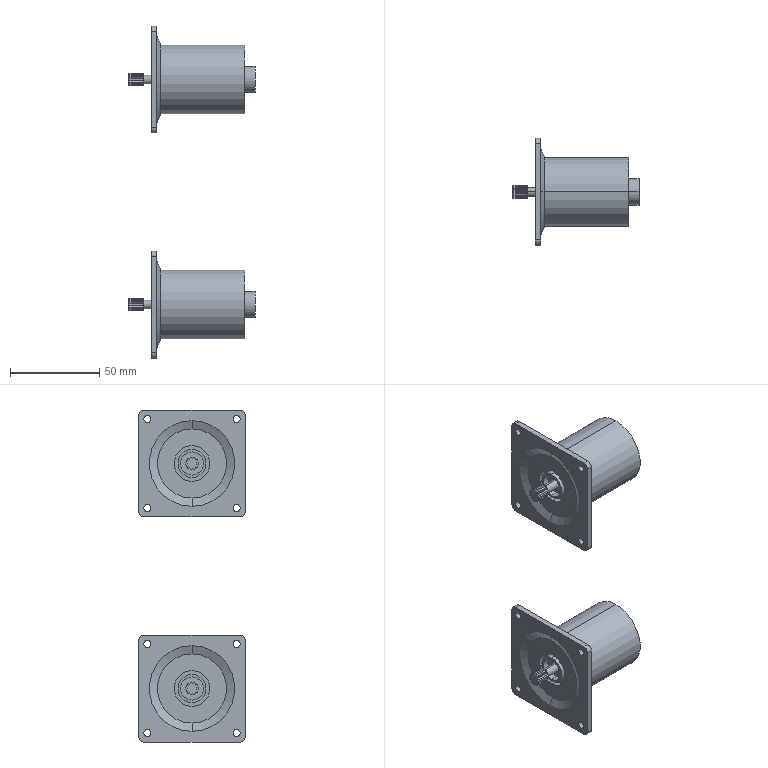Part | SolidWorks | features BaseBody 2 | 2 solids | 152 faces | box 70.7 x 60 x 186.2 mm | volume 133005 mm3 | plane 74 | cylinder 70 | cone 8 | commonest cylinder face diameters 7 x22 4 x16 6 x8 5 x4 13 x4 14.6 x4